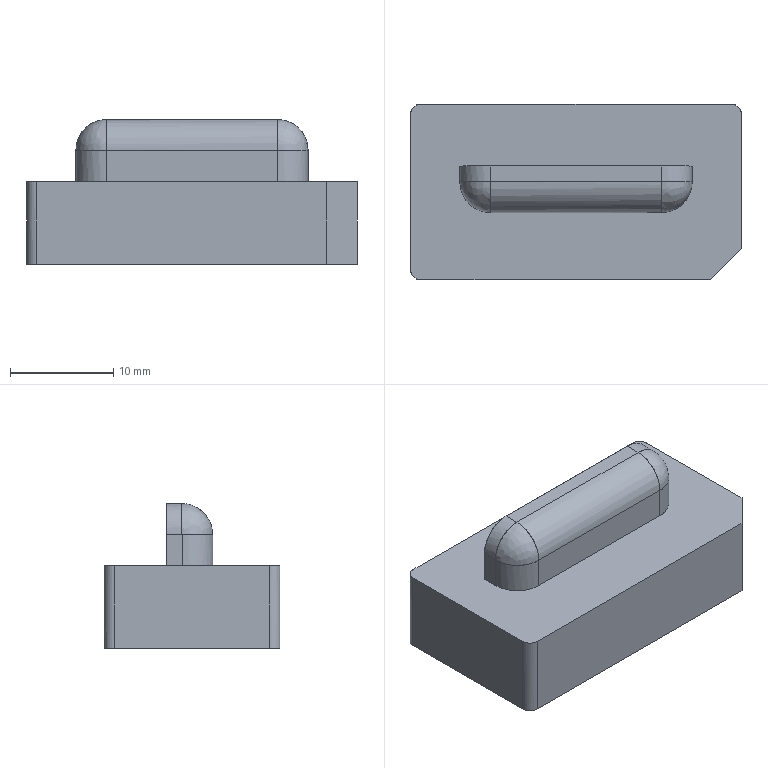CAM job | PowerMill | 3-axis milling, other | part box 32 x 17 x 14 mm
Tools:
number,name,type,diameter,tip_radius,length,cutting_length,overhang,flutes,holder,toolpaths_using
1,D10C,end_mill,10.0,0.0,60.0,,30.0,1,D42L35,1
1,D10C_1_1,end_mill,10.0,0.0,60.0,,14.44,1,D42L35,3
2,D4C_1_1,end_mill,4.0,0.0,30.0,,6.2,1,D42L35,2
3,D10_1_1,end_mill,10.0,0.0,60.0,,14.16,1,D42L35,2
22,R1.5_1_1,ball_nosed,3.0,1.5,30.0,,4.88,1,D42L35,1
10,D3_1_1,end_mill,3.0,0.0,30.0,,6.24,1,D42L35,1
13,Text_D4_1_1,taper_spherical,4.0,0.3,60.0,,6.24,1,D42L35,1
Operations:
program,toolpath,strategy,tool,tool_number,tool_diameter,tip_radius,flutes,spindle_rpm,feed_cut,surface_speed_m_min_computed,feed_per_tooth_computed,tolerance,thickness,stepover,stepdown,cut_length,cut_time_min,total_time_min,workplane
27-C01-8-F,精公开粗01-扫面平行-D10C,raster_area_clear,D10C_1_1,1,10.0,0.0,1.0,8000.0,10000.0,251.33,1.25,0.03,0.28,6.0,1.0,210.36,0.021,0.0268,
27-C01-8-F,精公开粗01-外形偏置-D10C,offset_area_clear,D10C_1_1,1,10.0,0.0,1.0,8000.0,10000.0,251.33,1.25,0.03,0.28,6.0,1.0,3120.468,0.312,0.3507,
27-C01-8-F,精公开粗01-基准台等高-D10C,constantz,D10C_1_1,1,10.0,0.0,1.0,8000.0,10000.0,251.33,1.25,0.03,0.07,5.0,0.4,2789.09,0.279,0.2874,
27-C01-8-F,精公再粗02-外形偏置-D4C,offset_area_clear,D4C_1_1,2,4.0,0.0,1.0,18000.0,6000.0,226.19,0.3333,0.03,0.0,2.0,1.0,2123.992,0.354,0.3711,
27-C01-8-F,精公再粗02-平行中光-D4C,raster,D4C_1_1,2,4.0,0.0,1.0,18000.0,6000.0,226.19,0.3333,0.03,0.0,0.2,1.0,1193.861,0.199,0.2083,
27-C01-8-F,精公基准台01-基准面偏置-D10,offset_area_clear,D10_1_1,3,10.0,0.0,1.0,8500.0,600.0,267.04,0.0706,0.005,0.38,5.0,1.0,96.021,0.16,0.178,
27-C01-8-F,精公基准台01-基准台侧光-D10,profile_area_clear,D10_1_1,3,10.0,0.0,1.0,8500.0,600.0,267.04,0.0706,0.005,0.0,0.08,1.0,253.233,0.422,0.4851,
27-C01-8-F,精公精光01-平行-R1.5,raster,R1.5_1_1,22,3.0,1.5,1.0,22000.0,2000.0,207.35,0.0909,0.005,-0.075,0.04,1.0,5733.069,2.866,2.909,
27-C01-8-F,精公精光02-等高-D3,constantz,D3_1_1,10,3.0,0.0,1.0,18000.0,2000.0,169.65,0.1111,0.005,-0.075,5.0,0.07,5157.114,2.579,2.584,
27-C01-8-F,精公刻字01-刻字-Text_D4,pattern,Text_D4_1_1,13,4.0,0.3,1.0,15000.0,1000.0,188.5,0.0667,0.005,0.0,5.0,1.0,52.321,0.052,0.0699,
,精公开粗01-外形偏置-D10C_Reference,offset_area_clear,D10C,1,10.0,0.0,1.0,8000.0,10000.0,251.33,1.25,0.03,0.28,6.0,1.0,6236.08,0.624,0.6987,